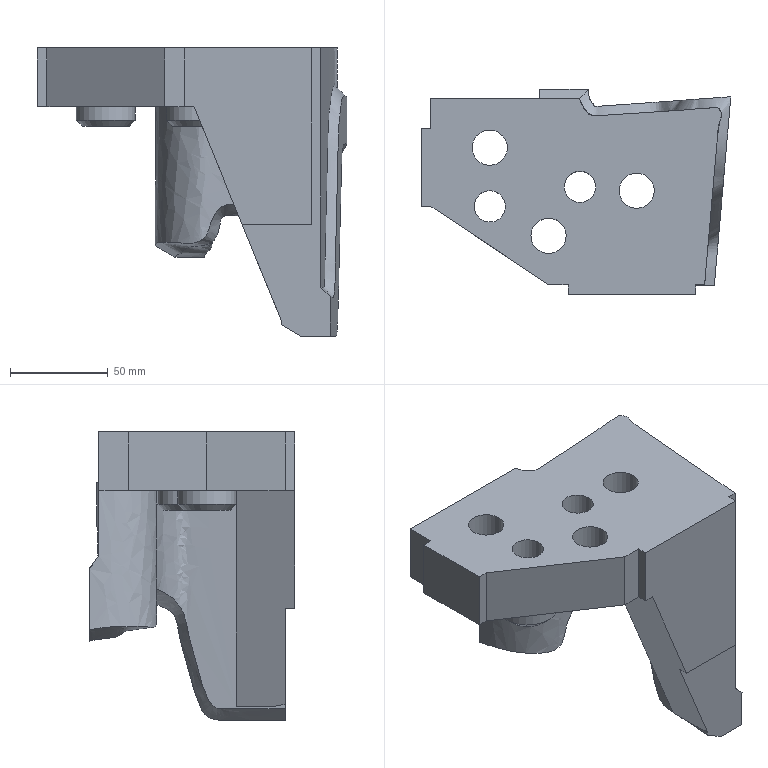Part | NX | features solid 2 | 1 solid | 45 faces | box 158 x 104.999 x 147.134 mm | volume 701592 mm3 | plane 25 | cylinder 10 | spline 8 | cone 2 | commonest cylinder face diameters 18 x3 26 x3 16 x2 30 x2